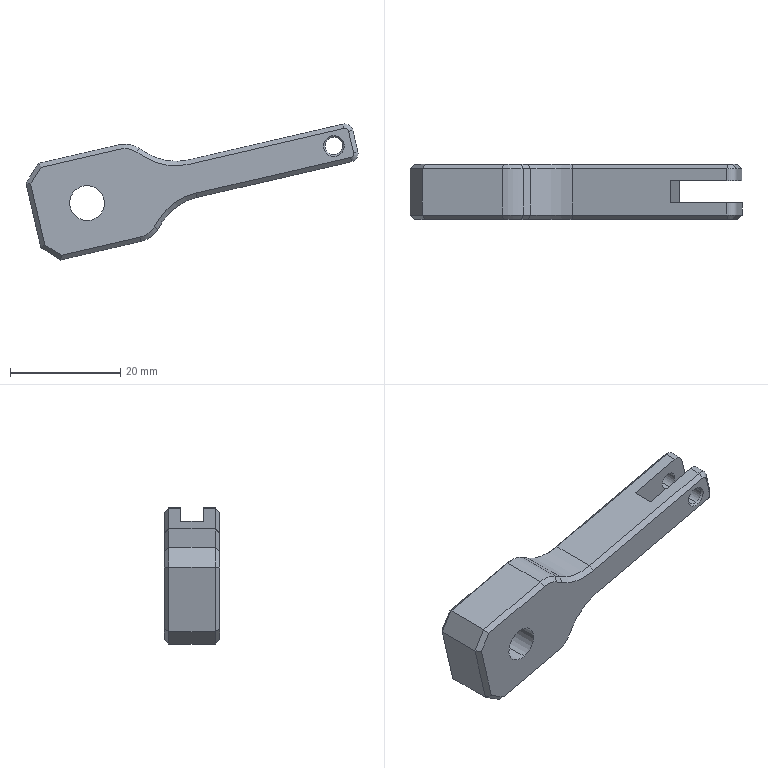Part | STEP file | 4-20.sldasm-Part-204 | 1 solid | 66 faces | box 60.3 x 10 x 24.703 mm | volume 5847 mm3 | plane 36 | cone 16 | cylinder 14 | commonest cylinder face diameters 3 x4 3.175 x4 6.35 x2 10 x2 20 x2